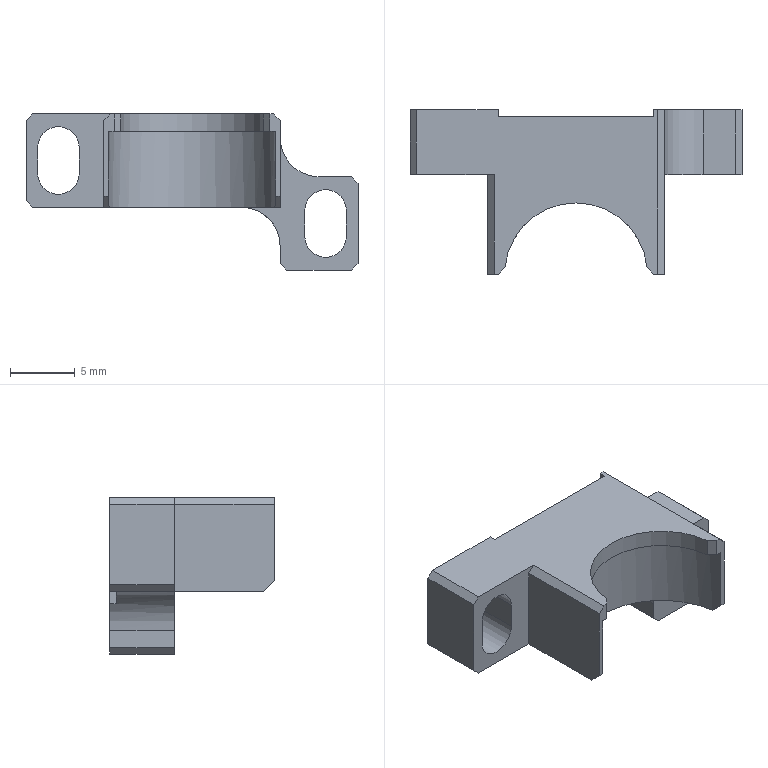Part | SolidWorks | features ICE 7, Chamfer 4, MoveFace 2, Extrusion 1, Fillet 1 | 1 solid | 42 faces | box 25.6 x 12.7 x 12.05 mm | volume 1054 mm3 | plane 34 | cylinder 8 | commonest cylinder face diameters 3.2 x4 6 x2 11 x1 12.9 x1
STEP:
#1=CARTESIAN_POINT('',(6.3,12.7,6.85));
#2=VERTEX_POINT('',#1);
#3=CARTESIAN_POINT('',(6.,12.7,6.85));
#4=VERTEX_POINT('',#3);
#5=CARTESIAN_POINT('',(0.,12.7,6.85));
#6=DIRECTION('',(-1.,0.,0.));
#7=VECTOR('',#6,1000.);
#8=LINE('',#5,#7);
#9=EDGE_CURVE('',#2,#4,#8,.T.);
#10=ORIENTED_EDGE('',*,*,#9,.F.);
#11=CARTESIAN_POINT('',(6.8,12.7,6.35));
#12=VERTEX_POINT('',#11);
#13=CARTESIAN_POINT('',(9.975,12.7,3.175));
#14=DIRECTION('',(0.7071,0.,-0.7071));
#15=VECTOR('',#14,1000.);
#16=LINE('',#13,#15);
#17=EDGE_CURVE('',#2,#12,#16,.T.);
#18=ORIENTED_EDGE('',*,*,#17,.T.);
#19=CARTESIAN_POINT('',(6.8,12.7,5.));
#20=VERTEX_POINT('',#19);
#21=CARTESIAN_POINT('',(6.8,12.7,0.));
#22=DIRECTION('',(0.,0.,1.));
#23=VECTOR('',#22,1000.);
#24=LINE('',#21,#23);
#25=EDGE_CURVE('',#20,#12,#24,.T.);
#26=ORIENTED_EDGE('',*,*,#25,.F.);
#27=CARTESIAN_POINT('',(9.8,12.7,2.));
#28=VERTEX_POINT('',#27);
#29=CARTESIAN_POINT('',(9.8,12.7,5.));
#30=DIRECTION('',(0.,-1.,0.));
#31=DIRECTION('',(-1.,0.,0.));
#32=AXIS2_PLACEMENT_3D('',#29,#30,#31);
#33=CIRCLE('',#32,3.);
#34=EDGE_CURVE('',#20,#28,#33,.T.);
#35=ORIENTED_EDGE('',*,*,#34,.T.);
#36=CARTESIAN_POINT('',(12.295,12.7,2.));
#37=VERTEX_POINT('',#36);
#38=CARTESIAN_POINT('',(6.8,12.7,2.));
#39=DIRECTION('',(1.,0.,0.));
#40=VECTOR('',#39,1000.);
#41=LINE('',#38,#40);
#42=EDGE_CURVE('',#28,#37,#41,.T.);
#43=ORIENTED_EDGE('',*,*,#42,.T.);
#44=CARTESIAN_POINT('',(12.8,12.7,1.495));
#45=VERTEX_POINT('',#44);
#46=CARTESIAN_POINT('',(10.547,12.7,3.747));
#47=DIRECTION('',(0.7071,0.,-0.7071));
#48=VECTOR('',#47,1000.);
#49=LINE('',#46,#48);
#50=EDGE_CURVE('',#37,#45,#49,.T.);
#51=ORIENTED_EDGE('',*,*,#50,.T.);
#52=CARTESIAN_POINT('',(12.8,12.7,-4.695));
#53=VERTEX_POINT('',#52);
#54=CARTESIAN_POINT('',(12.8,12.7,-5.2));
#55=DIRECTION('',(0.,0.,-1.));
#56=VECTOR('',#55,1000.);
#57=LINE('',#54,#56);
#58=EDGE_CURVE('',#45,#53,#57,.T.);
#59=ORIENTED_EDGE('',*,*,#58,.T.);
#60=CARTESIAN_POINT('',(12.295,12.7,-5.2));
#61=VERTEX_POINT('',#60);
#62=CARTESIAN_POINT('',(12.147,12.7,-5.347));
#63=DIRECTION('',(-0.7071,0.,-0.7071));
#64=VECTOR('',#63,1000.);
#65=LINE('',#62,#64);
#66=EDGE_CURVE('',#53,#61,#65,.T.);
#67=ORIENTED_EDGE('',*,*,#66,.T.);
#68=CARTESIAN_POINT('',(7.3,12.7,-5.2));
#69=VERTEX_POINT('',#68);
#70=CARTESIAN_POINT('',(6.8,12.7,-5.2));
#71=DIRECTION('',(-1.,0.,0.));
#72=VECTOR('',#71,1000.);
#73=LINE('',#70,#72);
#74=EDGE_CURVE('',#61,#69,#73,.T.);
#75=ORIENTED_EDGE('',*,*,#74,.T.);
#76=CARTESIAN_POINT('',(6.8,12.7,-4.7));
#77=VERTEX_POINT('',#76);
#78=CARTESIAN_POINT('',(4.45,12.7,-2.35));
#79=DIRECTION('',(-0.7071,0.,0.7071));
#80=VECTOR('',#79,1000.);
#81=LINE('',#78,#80);
#82=EDGE_CURVE('',#69,#77,#81,.T.);
#83=ORIENTED_EDGE('',*,*,#82,.T.);
#84=CARTESIAN_POINT('',(6.8,12.7,-3.35));
#85=VERTEX_POINT('',#84);
#86=CARTESIAN_POINT('',(6.8,12.7,-5.2));
#87=DIRECTION('',(0.,0.,1.));
#88=VECTOR('',#87,1000.);
#89=LINE('',#86,#88);
#90=EDGE_CURVE('',#77,#85,#89,.T.);
#91=ORIENTED_EDGE('',*,*,#90,.T.);
#92=CARTESIAN_POINT('',(6.,12.7,-1.31));
#93=VERTEX_POINT('',#92);
#94=CARTESIAN_POINT('',(3.8,12.7,-3.35));
#95=DIRECTION('',(0.,-1.,0.));
#96=DIRECTION('',(-1.,0.,0.));
#97=AXIS2_PLACEMENT_3D('',#94,#95,#96);
#98=CIRCLE('',#97,3.);
#99=EDGE_CURVE('',#85,#93,#98,.T.);
#100=ORIENTED_EDGE('',*,*,#99,.T.);
#101=CARTESIAN_POINT('',(6.,12.7,0.));
#102=DIRECTION('',(0.,0.,-1.));
#103=VECTOR('',#102,1000.);
#104=LINE('',#101,#103);
#105=EDGE_CURVE('',#4,#93,#104,.T.);
#106=ORIENTED_EDGE('',*,*,#105,.F.);
#107=EDGE_LOOP('',(#10,#18,#26,#35,#43,#51,#59,#67,#75,#83,#91,#100,#106));
#108=FACE_OUTER_BOUND('',#107,.T.);
#109=CARTESIAN_POINT('',(8.7,12.7,-2.6));
#110=VERTEX_POINT('',#109);
#111=CARTESIAN_POINT('',(11.9,12.7,-2.6));
#112=VERTEX_POINT('',#111);
#113=CARTESIAN_POINT('',(10.3,12.7,-2.6));
#114=DIRECTION('',(0.,-1.,0.));
#115=DIRECTION('',(1.,0.,0.));
#116=AXIS2_PLACEMENT_3D('',#113,#114,#115);
#117=CIRCLE('',#116,1.6);
#118=EDGE_CURVE('',#110,#112,#117,.T.);
#119=ORIENTED_EDGE('',*,*,#118,.T.);
#120=CARTESIAN_POINT('',(11.9,12.7,-0.6));
#121=VERTEX_POINT('',#120);
#122=CARTESIAN_POINT('',(11.9,12.7,-2.6));
#123=DIRECTION('',(0.,0.,1.));
#124=VECTOR('',#123,1000.);
#125=LINE('',#122,#124);
#126=EDGE_CURVE('',#112,#121,#125,.T.);
#127=ORIENTED_EDGE('',*,*,#126,.T.);
#128=CARTESIAN_POINT('',(8.7,12.7,-0.6));
#129=VERTEX_POINT('',#128);
#130=CARTESIAN_POINT('',(10.3,12.7,-0.6));
#131=DIRECTION('',(0.,-1.,0.));
#132=DIRECTION('',(1.,0.,0.));
#133=AXIS2_PLACEMENT_3D('',#130,#131,#132);
#134=CIRCLE('',#133,1.6);
#135=EDGE_CURVE('',#121,#129,#134,.T.);
#136=ORIENTED_EDGE('',*,*,#135,.T.);
#137=CARTESIAN_POINT('',(8.7,12.7,-2.6));
#138=DIRECTION('',(0.,0.,-1.));
#139=VECTOR('',#138,1000.);
#140=LINE('',#137,#139);
#141=EDGE_CURVE('',#129,#110,#140,.T.);
#142=ORIENTED_EDGE('',*,*,#141,.T.);
#143=EDGE_LOOP('',(#119,#127,#136,#142));
#144=FACE_BOUND('',#143,.T.);
#145=CARTESIAN_POINT('',(6.8,12.7,0.));
#146=DIRECTION('',(0.,1.,0.));
#147=DIRECTION('',(-1.,0.,0.));
#148=AXIS2_PLACEMENT_3D('',#145,#146,#147);
#149=PLANE('',#148);
#150=ADVANCED_FACE('',(#108,#144),#149,.T.);
#151=CARTESIAN_POINT('',(-6.8,0.,0.5));
#152=VERTEX_POINT('',#151);
#153=CARTESIAN_POINT('',(-6.8,0.,6.35));
#154=VERTEX_POINT('',#153);
#155=CARTESIAN_POINT('',(-6.8,0.,0.));
#156=DIRECTION('',(0.,0.,1.));
#157=VECTOR('',#156,1000.);
#158=LINE('',#155,#157);
#159=EDGE_CURVE('',#152,#154,#158,.T.);
#160=ORIENTED_EDGE('',*,*,#159,.T.);
#161=CARTESIAN_POINT('',(-6.8,7.7,6.35));
#162=VERTEX_POINT('',#161);
#163=CARTESIAN_POINT('',(-6.8,0.,6.35));
#164=DIRECTION('',(0.,1.,0.));
#165=VECTOR('',#164,1000.);
#166=LINE('',#163,#165);
#167=EDGE_CURVE('',#154,#162,#166,.T.);
#168=ORIENTED_EDGE('',*,*,#167,.T.);
#169=CARTESIAN_POINT('',(-6.8,7.7,-0.35));
#170=VERTEX_POINT('',#169);
#171=CARTESIAN_POINT('',(-6.8,7.7,6.5));
#172=DIRECTION('',(0.,0.,-1.));
#173=VECTOR('',#172,1000.);
#174=LINE('',#171,#173);
#175=EDGE_CURVE('',#162,#170,#174,.T.);
#176=ORIENTED_EDGE('',*,*,#175,.T.);
#177=CARTESIAN_POINT('',(-6.8,0.85,-0.35));
#178=VERTEX_POINT('',#177);
#179=CARTESIAN_POINT('',(-6.8,0.,-0.35));
#180=DIRECTION('',(0.,-1.,0.));
#181=VECTOR('',#180,1000.);
#182=LINE('',#179,#181);
#183=EDGE_CURVE('',#170,#178,#182,.T.);
#184=ORIENTED_EDGE('',*,*,#183,.T.);
#185=CARTESIAN_POINT('',(-6.8,0.25,0.25));
#186=DIRECTION('',(0.,-0.7071,0.7071));
#187=VECTOR('',#186,1000.);
#188=LINE('',#185,#187);
#189=EDGE_CURVE('',#178,#152,#188,.T.);
#190=ORIENTED_EDGE('',*,*,#189,.T.);
#191=EDGE_LOOP('',(#160,#168,#176,#184,#190));
#192=FACE_OUTER_BOUND('',#191,.T.);
#193=CARTESIAN_POINT('',(-6.8,0.,0.));
#194=DIRECTION('',(-1.,0.,0.));
#195=DIRECTION('',(0.,0.,1.));
#196=AXIS2_PLACEMENT_3D('',#193,#194,#195);
#197=PLANE('',#196);
#198=ADVANCED_FACE('',(#192),#197,.T.);
#199=CARTESIAN_POINT('',(5.475,0.5251,5.5));
#200=VERTEX_POINT('',#199);
#201=CARTESIAN_POINT('',(-5.475,0.5251,5.5));
#202=VERTEX_POINT('',#201);
#203=CARTESIAN_POINT('',(0.,0.,5.5));
#204=DIRECTION('',(0.,0.,1.));
#205=DIRECTION('',(-1.,0.,0.));
#206=AXIS2_PLACEMENT_3D('',#203,#204,#205);
#207=CIRCLE('',#206,5.5);
#208=EDGE_CURVE('',#200,#202,#207,.T.);
#209=ORIENTED_EDGE('',*,*,#208,.F.);
#210=CARTESIAN_POINT('',(5.475,0.5251,6.85));
#211=VERTEX_POINT('',#210);
#212=CARTESIAN_POINT('',(5.475,0.5251,10.));
#213=DIRECTION('',(0.,0.,1.));
#214=VECTOR('',#213,1000.);
#215=LINE('',#212,#214);
#216=EDGE_CURVE('',#200,#211,#215,.T.);
#217=ORIENTED_EDGE('',*,*,#216,.T.);
#218=CARTESIAN_POINT('',(-5.475,0.5251,6.85));
#219=VERTEX_POINT('',#218);
#220=CARTESIAN_POINT('',(0.,0.,6.85));
#221=DIRECTION('',(0.,0.,1.));
#222=DIRECTION('',(1.,0.,0.));
#223=AXIS2_PLACEMENT_3D('',#220,#221,#222);
#224=CIRCLE('',#223,5.5);
#225=EDGE_CURVE('',#211,#219,#224,.T.);
#226=ORIENTED_EDGE('',*,*,#225,.T.);
#227=CARTESIAN_POINT('',(-5.475,0.5251,10.));
#228=DIRECTION('',(0.,0.,-1.));
#229=VECTOR('',#228,1000.);
#230=LINE('',#227,#229);
#231=EDGE_CURVE('',#219,#202,#230,.T.);
#232=ORIENTED_EDGE('',*,*,#231,.T.);
#233=EDGE_LOOP('',(#209,#217,#226,#232));
#234=FACE_OUTER_BOUND('',#233,.T.);
#235=CARTESIAN_POINT('',(0.,0.,10.));
#236=DIRECTION('',(0.,0.,-1.));
#237=DIRECTION('',(-1.,0.,0.));
#238=AXIS2_PLACEMENT_3D('',#235,#236,#237);
#239=CYLINDRICAL_SURFACE('',#238,5.5);
#240=ADVANCED_FACE('',(#234),#239,.F.);
#241=CARTESIAN_POINT('',(-12.3,7.7,6.85));
#242=VERTEX_POINT('',#241);
#243=CARTESIAN_POINT('',(-6.3,7.7,6.85));
#244=VERTEX_POINT('',#243);
#245=CARTESIAN_POINT('',(0.,7.7,6.85));
#246=DIRECTION('',(1.,0.,0.));
#247=VECTOR('',#246,1000.);
#248=LINE('',#245,#247);
#249=EDGE_CURVE('',#242,#244,#248,.T.);
#250=ORIENTED_EDGE('',*,*,#249,.T.);
#251=CARTESIAN_POINT('',(-6.3,0.,6.85));
#252=VERTEX_POINT('',#251);
#253=CARTESIAN_POINT('',(-6.3,0.,6.85));
#254=DIRECTION('',(0.,-1.,0.));
#255=VECTOR('',#254,1000.);
#256=LINE('',#253,#255);
#257=EDGE_CURVE('',#244,#252,#256,.T.);
#258=ORIENTED_EDGE('',*,*,#257,.T.);
#259=CARTESIAN_POINT('',(-6.,0.,6.85));
#260=VERTEX_POINT('',#259);
#261=CARTESIAN_POINT('',(0.,0.,6.85));
#262=DIRECTION('',(-1.,0.,0.));
#263=VECTOR('',#262,1000.);
#264=LINE('',#261,#263);
#265=EDGE_CURVE('',#260,#252,#264,.T.);
#266=ORIENTED_EDGE('',*,*,#265,.F.);
#267=CARTESIAN_POINT('',(-3.,3.,6.85));
#268=DIRECTION('',(0.7071,0.7071,0.));
#269=VECTOR('',#268,1000.);
#270=LINE('',#267,#269);
#271=EDGE_CURVE('',#260,#219,#270,.T.);
#272=ORIENTED_EDGE('',*,*,#271,.T.);
#273=ORIENTED_EDGE('',*,*,#225,.F.);
#274=CARTESIAN_POINT('',(6.,0.,6.85));
#275=VERTEX_POINT('',#274);
#276=CARTESIAN_POINT('',(3.,3.,6.85));
#277=DIRECTION('',(0.7071,-0.7071,0.));
#278=VECTOR('',#277,1000.);
#279=LINE('',#276,#278);
#280=EDGE_CURVE('',#211,#275,#279,.T.);
#281=ORIENTED_EDGE('',*,*,#280,.T.);
#282=CARTESIAN_POINT('',(6.3,0.,6.85));
#283=VERTEX_POINT('',#282);
#284=CARTESIAN_POINT('',(0.,0.,6.85));
#285=DIRECTION('',(-1.,0.,0.));
#286=VECTOR('',#285,1000.);
#287=LINE('',#284,#286);
#288=EDGE_CURVE('',#283,#275,#287,.T.);
#289=ORIENTED_EDGE('',*,*,#288,.F.);
#290=CARTESIAN_POINT('',(6.3,0.,6.85));
#291=DIRECTION('',(0.,1.,0.));
#292=VECTOR('',#291,1000.);
#293=LINE('',#290,#292);
#294=EDGE_CURVE('',#283,#2,#293,.T.);
#295=ORIENTED_EDGE('',*,*,#294,.T.);
#296=ORIENTED_EDGE('',*,*,#9,.T.);
#297=CARTESIAN_POINT('',(6.,12.2,6.85));
#298=VERTEX_POINT('',#297);
#299=CARTESIAN_POINT('',(6.,0.,6.85));
#300=DIRECTION('',(0.,1.,0.));
#301=VECTOR('',#300,1000.);
#302=LINE('',#299,#301);
#303=EDGE_CURVE('',#298,#4,#302,.T.);
#304=ORIENTED_EDGE('',*,*,#303,.F.);
#305=CARTESIAN_POINT('',(-6.,12.2,6.85));
#306=VERTEX_POINT('',#305);
#307=CARTESIAN_POINT('',(0.,12.2,6.85));
#308=DIRECTION('',(1.,0.,0.));
#309=VECTOR('',#308,1000.);
#310=LINE('',#307,#309);
#311=EDGE_CURVE('',#306,#298,#310,.T.);
#312=ORIENTED_EDGE('',*,*,#311,.F.);
#313=CARTESIAN_POINT('',(-6.,12.7,6.85));
#314=VERTEX_POINT('',#313);
#315=CARTESIAN_POINT('',(-6.,12.2,6.85));
#316=DIRECTION('',(0.,1.,0.));
#317=VECTOR('',#316,1000.);
#318=LINE('',#315,#317);
#319=EDGE_CURVE('',#306,#314,#318,.T.);
#320=ORIENTED_EDGE('',*,*,#319,.T.);
#321=CARTESIAN_POINT('',(-12.3,12.7,6.85));
#322=VERTEX_POINT('',#321);
#323=CARTESIAN_POINT('',(0.,12.7,6.85));
#324=DIRECTION('',(-1.,0.,0.));
#325=VECTOR('',#324,1000.);
#326=LINE('',#323,#325);
#327=EDGE_CURVE('',#314,#322,#326,.T.);
#328=ORIENTED_EDGE('',*,*,#327,.T.);
#329=CARTESIAN_POINT('',(-12.3,0.,6.85));
#330=DIRECTION('',(0.,-1.,0.));
#331=VECTOR('',#330,1000.);
#332=LINE('',#329,#331);
#333=EDGE_CURVE('',#322,#242,#332,.T.);
#334=ORIENTED_EDGE('',*,*,#333,.T.);
#335=EDGE_LOOP('',(#250,#258,#266,#272,#273,#281,#289,#295,#296,#304,#312,#320,#328,#334));
#336=FACE_OUTER_BOUND('',#335,.T.);
#337=CARTESIAN_POINT('',(0.,0.,6.85));
#338=DIRECTION('',(0.,0.,1.));
#339=DIRECTION('',(1.,0.,0.));
#340=AXIS2_PLACEMENT_3D('',#337,#338,#339);
#341=PLANE('',#340);
#342=ADVANCED_FACE('',(#336),#341,.T.);
#343=CARTESIAN_POINT('',(-12.3,7.7,-0.35));
#344=VERTEX_POINT('',#343);
#345=CARTESIAN_POINT('',(0.,7.7,-0.35));
#346=DIRECTION('',(-1.,0.,0.));
#347=VECTOR('',#346,1000.);
#348=LINE('',#345,#347);
#349=EDGE_CURVE('',#170,#344,#348,.T.);
#350=ORIENTED_EDGE('',*,*,#349,.T.);
#351=CARTESIAN_POINT('',(-12.3,12.7,-0.35));
#352=VERTEX_POINT('',#351);
#353=CARTESIAN_POINT('',(-12.3,12.7,-0.35));
#354=DIRECTION('',(0.,1.,0.));
#355=VECTOR('',#354,1000.);
#356=LINE('',#353,#355);
#357=EDGE_CURVE('',#344,#352,#356,.T.);
#358=ORIENTED_EDGE('',*,*,#357,.T.);
#359=CARTESIAN_POINT('',(-6.,12.7,-0.35));
#360=VERTEX_POINT('',#359);
#361=CARTESIAN_POINT('',(0.,12.7,-0.35));
#362=DIRECTION('',(-1.,0.,0.));
#363=VECTOR('',#362,1000.);
#364=LINE('',#361,#363);
#365=EDGE_CURVE('',#360,#352,#364,.T.);
#366=ORIENTED_EDGE('',*,*,#365,.F.);
#367=CARTESIAN_POINT('',(-6.,12.2,-0.35));
#368=VERTEX_POINT('',#367);
#369=CARTESIAN_POINT('',(-6.,12.2,-0.35));
#370=DIRECTION('',(0.,1.,0.));
#371=VECTOR('',#370,1000.);
#372=LINE('',#369,#371);
#373=EDGE_CURVE('',#368,#360,#372,.T.);
#374=ORIENTED_EDGE('',*,*,#373,.F.);
#375=CARTESIAN_POINT('',(3.8,12.2,-0.35));
#376=VERTEX_POINT('',#375);
#377=CARTESIAN_POINT('',(0.,12.2,-0.35));
#378=DIRECTION('',(-1.,0.,0.));
#379=VECTOR('',#378,1000.);
#380=LINE('',#377,#379);
#381=EDGE_CURVE('',#376,#368,#380,.T.);
#382=ORIENTED_EDGE('',*,*,#381,.F.);
#383=CARTESIAN_POINT('',(3.8,7.7,-0.35));
#384=VERTEX_POINT('',#383);
#385=CARTESIAN_POINT('',(3.8,0.,-0.35));
#386=DIRECTION('',(0.,-1.,0.));
#387=VECTOR('',#386,1000.);
#388=LINE('',#385,#387);
#389=EDGE_CURVE('',#376,#384,#388,.T.);
#390=ORIENTED_EDGE('',*,*,#389,.T.);
#391=CARTESIAN_POINT('',(6.8,7.7,-0.35));
#392=VERTEX_POINT('',#391);
#393=CARTESIAN_POINT('',(0.,7.7,-0.35));
#394=DIRECTION('',(1.,0.,0.));
#395=VECTOR('',#394,1000.);
#396=LINE('',#393,#395);
#397=EDGE_CURVE('',#384,#392,#396,.T.);
#398=ORIENTED_EDGE('',*,*,#397,.T.);
#399=CARTESIAN_POINT('',(6.8,0.85,-0.35));
#400=VERTEX_POINT('',#399);
#401=CARTESIAN_POINT('',(6.8,0.,-0.35));
#402=DIRECTION('',(0.,1.,0.));
#403=VECTOR('',#402,1000.);
#404=LINE('',#401,#403);
#405=EDGE_CURVE('',#400,#392,#404,.T.);
#406=ORIENTED_EDGE('',*,*,#405,.F.);
#407=CARTESIAN_POINT('',(6.394,0.85,-0.35));
#408=VERTEX_POINT('',#407);
#409=CARTESIAN_POINT('',(-6.8,0.85,-0.35));
#410=DIRECTION('',(-1.,0.,0.));
#411=VECTOR('',#410,1000.);
#412=LINE('',#409,#411);
#413=EDGE_CURVE('',#400,#408,#412,.T.);
#414=ORIENTED_EDGE('',*,*,#413,.T.);
#415=CARTESIAN_POINT('',(-6.394,0.85,-0.35));
#416=VERTEX_POINT('',#415);
#417=CARTESIAN_POINT('',(0.,0.,-0.35));
#418=DIRECTION('',(0.,0.,-1.));
#419=DIRECTION('',(1.,0.,0.));
#420=AXIS2_PLACEMENT_3D('',#417,#418,#419);
#421=CIRCLE('',#420,6.45);
#422=EDGE_CURVE('',#416,#408,#421,.T.);
#423=ORIENTED_EDGE('',*,*,#422,.F.);
#424=CARTESIAN_POINT('',(-6.8,0.85,-0.35));
#425=DIRECTION('',(-1.,0.,0.));
#426=VECTOR('',#425,1000.);
#427=LINE('',#424,#426);
#428=EDGE_CURVE('',#416,#178,#427,.T.);
#429=ORIENTED_EDGE('',*,*,#428,.T.);
#430=ORIENTED_EDGE('',*,*,#183,.F.);
#431=EDGE_LOOP('',(#350,#358,#366,#374,#382,#390,#398,#406,#414,#423,#429,#430));
#432=FACE_OUTER_BOUND('',#431,.T.);
#433=CARTESIAN_POINT('',(0.,0.,-0.35));
#434=DIRECTION('',(0.,0.,1.));
#435=DIRECTION('',(1.,0.,0.));
#436=AXIS2_PLACEMENT_3D('',#433,#434,#435);
#437=PLANE('',#436);
#438=ADVANCED_FACE('',(#432),#437,.F.);
#439=CARTESIAN_POINT('',(6.,0.,5.5));
#440=VERTEX_POINT('',#439);
#441=CARTESIAN_POINT('',(6.45,0.,5.5));
#442=VERTEX_POINT('',#441);
#443=CARTESIAN_POINT('',(0.,0.,5.5));
#444=DIRECTION('',(1.,0.,0.));
#445=VECTOR('',#444,1000.);
#446=LINE('',#443,#445);
#447=EDGE_CURVE('',#440,#442,#446,.T.);
#448=ORIENTED_EDGE('',*,*,#447,.F.);
#449=CARTESIAN_POINT('',(3.,3.,5.5));
#450=DIRECTION('',(-0.7071,0.7071,0.));
#451=VECTOR('',#450,1000.);
#452=LINE('',#449,#451);
#453=EDGE_CURVE('',#440,#200,#452,.T.);
#454=ORIENTED_EDGE('',*,*,#453,.T.);
#455=ORIENTED_EDGE('',*,*,#208,.T.);
#456=CARTESIAN_POINT('',(-6.,0.,5.5));
#457=VERTEX_POINT('',#456);
#458=CARTESIAN_POINT('',(-3.,3.,5.5));
#459=DIRECTION('',(-0.7071,-0.7071,0.));
#460=VECTOR('',#459,1000.);
#461=LINE('',#458,#460);
#462=EDGE_CURVE('',#202,#457,#461,.T.);
#463=ORIENTED_EDGE('',*,*,#462,.T.);
#464=CARTESIAN_POINT('',(-6.45,0.,5.5));
#465=VERTEX_POINT('',#464);
#466=CARTESIAN_POINT('',(0.,0.,5.5));
#467=DIRECTION('',(1.,0.,0.));
#468=VECTOR('',#467,1000.);
#469=LINE('',#466,#468);
#470=EDGE_CURVE('',#465,#457,#469,.T.);
#471=ORIENTED_EDGE('',*,*,#470,.F.);
#472=CARTESIAN_POINT('',(0.,0.,5.5));
#473=DIRECTION('',(0.,0.,-1.));
#474=DIRECTION('',(-1.,0.,0.));
#475=AXIS2_PLACEMENT_3D('',#472,#473,#474);
#476=CIRCLE('',#475,6.45);
#477=EDGE_CURVE('',#465,#442,#476,.T.);
#478=ORIENTED_EDGE('',*,*,#477,.T.);
#479=EDGE_LOOP('',(#448,#454,#455,#463,#471,#478));
#480=FACE_OUTER_BOUND('',#479,.T.);
#481=CARTESIAN_POINT('',(0.,0.,5.5));
#482=DIRECTION('',(0.,0.,-1.));
#483=DIRECTION('',(-1.,0.,0.));
#484=AXIS2_PLACEMENT_3D('',#481,#482,#483);
#485=PLANE('',#484);
#486=ADVANCED_FACE('',(#480),#485,.T.);
#487=ORIENTED_EDGE('',*,*,#422,.T.);
#488=CARTESIAN_POINT('',(6.45,0.,0.5));
#489=VERTEX_POINT('',#488);
#490=CARTESIAN_POINT('',(6.394,0.85,-0.35));
#491=CARTESIAN_POINT('',(6.431,0.5681,-0.06811));
#492=CARTESIAN_POINT('',(6.45,0.2844,0.2156));
#493=CARTESIAN_POINT('',(6.45,0.,0.5));
#494=(BOUNDED_CURVE()B_SPLINE_CURVE(3,(#490,#491,#492,#493),.UNSPECIFIED.,.F.,.F.)B_SPLINE_CURVE_WITH_KNOTS((4,4),(1.439,1.571),.UNSPECIFIED.)CURVE()GEOMETRIC_REPRESENTATION_ITEM()RATIONAL_B_SPLINE_CURVE((1.,0.9985,0.9985,1.))REPRESENTATION_ITEM(''));
#495=EDGE_CURVE('',#408,#489,#494,.T.);
#496=ORIENTED_EDGE('',*,*,#495,.T.);
#497=CARTESIAN_POINT('',(6.45,0.,5.5));
#498=DIRECTION('',(0.,0.,1.));
#499=VECTOR('',#498,1000.);
#500=LINE('',#497,#499);
#501=EDGE_CURVE('',#489,#442,#500,.T.);
#502=ORIENTED_EDGE('',*,*,#501,.T.);
#503=ORIENTED_EDGE('',*,*,#477,.F.);
#504=CARTESIAN_POINT('',(-6.45,0.,0.5));
#505=VERTEX_POINT('',#504);
#506=CARTESIAN_POINT('',(-6.45,0.,5.5));
#507=DIRECTION('',(0.,0.,-1.));
#508=VECTOR('',#507,1000.);
#509=LINE('',#506,#508);
#510=EDGE_CURVE('',#465,#505,#509,.T.);
#511=ORIENTED_EDGE('',*,*,#510,.T.);
#512=CARTESIAN_POINT('',(-6.45,0.,0.5));
#513=CARTESIAN_POINT('',(-6.45,0.2844,0.2156));
#514=CARTESIAN_POINT('',(-6.431,0.5681,-0.06811));
#515=CARTESIAN_POINT('',(-6.394,0.85,-0.35));
#516=(BOUNDED_CURVE()B_SPLINE_CURVE(3,(#512,#513,#514,#515),.UNSPECIFIED.,.F.,.F.)B_SPLINE_CURVE_WITH_KNOTS((4,4),(4.712,4.845),.UNSPECIFIED.)CURVE()GEOMETRIC_REPRESENTATION_ITEM()RATIONAL_B_SPLINE_CURVE((1.,0.9985,0.9985,1.))REPRESENTATION_ITEM(''));
#517=EDGE_CURVE('',#505,#416,#516,.T.);
#518=ORIENTED_EDGE('',*,*,#517,.T.);
#519=EDGE_LOOP('',(#487,#496,#502,#503,#511,#518));
#520=FACE_OUTER_BOUND('',#519,.T.);
#521=CARTESIAN_POINT('',(0.,0.,5.5));
#522=DIRECTION('',(0.,0.,-1.));
#523=DIRECTION('',(-1.,0.,0.));
#524=AXIS2_PLACEMENT_3D('',#521,#522,#523);
#525=CYLINDRICAL_SURFACE('',#524,6.45);
#526=ADVANCED_FACE('',(#520),#525,.F.);
#527=CARTESIAN_POINT('',(-12.8,12.7,0.15));
#528=VERTEX_POINT('',#527);
#529=CARTESIAN_POINT('',(-12.8,12.7,6.35));
#530=VERTEX_POINT('',#529);
#531=CARTESIAN_POINT('',(-12.8,12.7,6.5));
#532=DIRECTION('',(0.,0.,1.));
#533=VECTOR('',#532,1000.);
#534=LINE('',#531,#533);
#535=EDGE_CURVE('',#528,#530,#534,.T.);
#536=ORIENTED_EDGE('',*,*,#535,.T.);
#537=CARTESIAN_POINT('',(-6.175,12.7,12.975));
#538=DIRECTION('',(0.7071,0.,0.7071));
#539=VECTOR('',#538,1000.);
#540=LINE('',#537,#539);
#541=EDGE_CURVE('',#530,#322,#540,.T.);
#542=ORIENTED_EDGE('',*,*,#541,.T.);
#543=ORIENTED_EDGE('',*,*,#327,.F.);
#544=CARTESIAN_POINT('',(-6.,12.7,6.5));
#545=DIRECTION('',(0.,0.,1.));
#546=VECTOR('',#545,1000.);
#547=LINE('',#544,#546);
#548=EDGE_CURVE('',#360,#314,#547,.T.);
#549=ORIENTED_EDGE('',*,*,#548,.F.);
#550=ORIENTED_EDGE('',*,*,#365,.T.);
#551=CARTESIAN_POINT('',(-2.925,12.7,-9.725));
#552=DIRECTION('',(-0.7071,0.,0.7071));
#553=VECTOR('',#552,1000.);
#554=LINE('',#551,#553);
#555=EDGE_CURVE('',#352,#528,#554,.T.);
#556=ORIENTED_EDGE('',*,*,#555,.T.);
#557=EDGE_LOOP('',(#536,#542,#543,#549,#550,#556));
#558=FACE_OUTER_BOUND('',#557,.T.);
#559=CARTESIAN_POINT('',(-8.7,12.7,4.25));
#560=VERTEX_POINT('',#559);
#561=CARTESIAN_POINT('',(-11.9,12.7,4.25));
#562=VERTEX_POINT('',#561);
#563=CARTESIAN_POINT('',(-10.3,12.7,4.25));
#564=DIRECTION('',(0.,-1.,0.));
#565=DIRECTION('',(-1.,0.,0.));
#566=AXIS2_PLACEMENT_3D('',#563,#564,#565);
#567=CIRCLE('',#566,1.6);
#568=EDGE_CURVE('',#560,#562,#567,.T.);
#569=ORIENTED_EDGE('',*,*,#568,.T.);
#570=CARTESIAN_POINT('',(-11.9,12.7,2.25));
#571=VERTEX_POINT('',#570);
#572=CARTESIAN_POINT('',(-11.9,12.7,2.25));
#573=DIRECTION('',(0.,0.,-1.));
#574=VECTOR('',#573,1000.);
#575=LINE('',#572,#574);
#576=EDGE_CURVE('',#562,#571,#575,.T.);
#577=ORIENTED_EDGE('',*,*,#576,.T.);
#578=CARTESIAN_POINT('',(-8.7,12.7,2.25));
#579=VERTEX_POINT('',#578);
#580=CARTESIAN_POINT('',(-10.3,12.7,2.25));
#581=DIRECTION('',(0.,-1.,0.));
#582=DIRECTION('',(-1.,0.,0.));
#583=AXIS2_PLACEMENT_3D('',#580,#581,#582);
#584=CIRCLE('',#583,1.6);
#585=EDGE_CURVE('',#571,#579,#584,.T.);
#586=ORIENTED_EDGE('',*,*,#585,.T.);
#587=CARTESIAN_POINT('',(-8.7,12.7,2.25));
#588=DIRECTION('',(0.,0.,1.));
#589=VECTOR('',#588,1000.);
#590=LINE('',#587,#589);
#591=EDGE_CURVE('',#579,#560,#590,.T.);
#592=ORIENTED_EDGE('',*,*,#591,.T.);
#593=EDGE_LOOP('',(#569,#577,#586,#592));
#594=FACE_BOUND('',#593,.T.);
#595=CARTESIAN_POINT('',(6.8,12.7,0.));
#596=DIRECTION('',(0.,1.,0.));
#597=DIRECTION('',(-1.,0.,0.));
#598=AXIS2_PLACEMENT_3D('',#595,#596,#597);
#599=PLANE('',#598);
#600=ADVANCED_FACE('',(#558,#594),#599,.T.);
#601=ORIENTED_EDGE('',*,*,#25,.T.);
#602=CARTESIAN_POINT('',(6.8,0.,6.35));
#603=VERTEX_POINT('',#602);
#604=CARTESIAN_POINT('',(6.8,0.,6.35));
#605=DIRECTION('',(0.,-1.,0.));
#606=VECTOR('',#605,1000.);
#607=LINE('',#604,#606);
#608=EDGE_CURVE('',#12,#603,#607,.T.);
#609=ORIENTED_EDGE('',*,*,#608,.T.);
#610=CARTESIAN_POINT('',(6.8,0.,0.5));
#611=VERTEX_POINT('',#610);
#612=CARTESIAN_POINT('',(6.8,0.,0.));
#613=DIRECTION('',(0.,0.,1.));
#614=VECTOR('',#613,1000.);
#615=LINE('',#612,#614);
#616=EDGE_CURVE('',#611,#603,#615,.T.);
#617=ORIENTED_EDGE('',*,*,#616,.F.);
#618=CARTESIAN_POINT('',(6.8,0.25,0.25));
#619=DIRECTION('',(0.,0.7071,-0.7071));
#620=VECTOR('',#619,1000.);
#621=LINE('',#618,#620);
#622=EDGE_CURVE('',#611,#400,#621,.T.);
#623=ORIENTED_EDGE('',*,*,#622,.T.);
#624=ORIENTED_EDGE('',*,*,#405,.T.);
#625=CARTESIAN_POINT('',(6.8,7.7,5.));
#626=VERTEX_POINT('',#625);
#627=CARTESIAN_POINT('',(6.8,7.7,0.));
#628=DIRECTION('',(0.,0.,1.));
#629=VECTOR('',#628,1000.);
#630=LINE('',#627,#629);
#631=EDGE_CURVE('',#392,#626,#630,.T.);
#632=ORIENTED_EDGE('',*,*,#631,.T.);
#633=CARTESIAN_POINT('',(6.8,12.7,5.));
#634=DIRECTION('',(0.,1.,0.));
#635=VECTOR('',#634,1000.);
#636=LINE('',#633,#635);
#637=EDGE_CURVE('',#626,#20,#636,.T.);
#638=ORIENTED_EDGE('',*,*,#637,.T.);
#639=EDGE_LOOP('',(#601,#609,#617,#623,#624,#632,#638));
#640=FACE_OUTER_BOUND('',#639,.T.);
#641=CARTESIAN_POINT('',(6.8,0.,0.));
#642=DIRECTION('',(1.,0.,0.));
#643=DIRECTION('',(0.,0.,-1.));
#644=AXIS2_PLACEMENT_3D('',#641,#642,#643);
#645=PLANE('',#644);
#646=ADVANCED_FACE('',(#640),#645,.T.);
#647=ORIENTED_EDGE('',*,*,#90,.F.);
#648=CARTESIAN_POINT('',(6.8,7.7,-4.7));
#649=VERTEX_POINT('',#648);
#650=CARTESIAN_POINT('',(6.8,7.7,-4.7));
#651=DIRECTION('',(0.,-1.,0.));
#652=VECTOR('',#651,1000.);
#653=LINE('',#650,#652);
#654=EDGE_CURVE('',#77,#649,#653,.T.);
#655=ORIENTED_EDGE('',*,*,#654,.T.);
#656=CARTESIAN_POINT('',(6.8,7.7,-3.35));
#657=VERTEX_POINT('',#656);
#658=CARTESIAN_POINT('',(6.8,7.7,-5.2));
#659=DIRECTION('',(0.,0.,1.));
#660=VECTOR('',#659,1000.);
#661=LINE('',#658,#660);
#662=EDGE_CURVE('',#649,#657,#661,.T.);
#663=ORIENTED_EDGE('',*,*,#662,.T.);
#664=CARTESIAN_POINT('',(6.8,7.7,-3.35));
#665=DIRECTION('',(0.,1.,0.));
#666=VECTOR('',#665,1000.);
#667=LINE('',#664,#666);
#668=EDGE_CURVE('',#657,#85,#667,.T.);
#669=ORIENTED_EDGE('',*,*,#668,.T.);
#670=EDGE_LOOP('',(#647,#655,#663,#669));
#671=FACE_OUTER_BOUND('',#670,.T.);
#672=CARTESIAN_POINT('',(6.8,7.7,-5.2));
#673=DIRECTION('',(-1.,0.,0.));
#674=DIRECTION('',(0.,-1.,0.));
#675=AXIS2_PLACEMENT_3D('',#672,#673,#674);
#676=PLANE('',#675);
#677=ADVANCED_FACE('',(#671),#676,.T.);
#678=CARTESIAN_POINT('',(12.295,7.7,-5.2));
#679=VERTEX_POINT('',#678);
#680=CARTESIAN_POINT('',(7.3,7.7,-5.2));
#681=VERTEX_POINT('',#680);
#682=CARTESIAN_POINT('',(6.8,7.7,-5.2));
#683=DIRECTION('',(-1.,0.,0.));
#684=VECTOR('',#683,1000.);
#685=LINE('',#682,#684);
#686=EDGE_CURVE('',#679,#681,#685,.T.);
#687=ORIENTED_EDGE('',*,*,#686,.T.);
#688=CARTESIAN_POINT('',(7.3,7.7,-5.2));
#689=DIRECTION('',(0.,1.,0.));
#690=VECTOR('',#689,1000.);
#691=LINE('',#688,#690);
#692=EDGE_CURVE('',#681,#69,#691,.T.);
#693=ORIENTED_EDGE('',*,*,#692,.T.);
#694=ORIENTED_EDGE('',*,*,#74,.F.);
#695=CARTESIAN_POINT('',(12.295,7.7,-5.2));
#696=DIRECTION('',(0.,-1.,0.));
#697=VECTOR('',#696,1000.);
#698=LINE('',#695,#697);
#699=EDGE_CURVE('',#61,#679,#698,.T.);
#700=ORIENTED_EDGE('',*,*,#699,.T.);
#701=EDGE_LOOP('',(#687,#693,#694,#700));
#702=FACE_OUTER_BOUND('',#701,.T.);
#703=CARTESIAN_POINT('',(6.8,7.7,-5.2));
#704=DIRECTION('',(0.,0.,-1.));
#705=DIRECTION('',(-1.,0.,0.));
#706=AXIS2_PLACEMENT_3D('',#703,#704,#705);
#707=PLANE('',#706);
#708=ADVANCED_FACE('',(#702),#707,.T.);
#709=CARTESIAN_POINT('',(12.8,7.7,1.495));
#710=VERTEX_POINT('',#709);
#711=CARTESIAN_POINT('',(12.8,7.7,-4.695));
#712=VERTEX_POINT('',#711);
#713=CARTESIAN_POINT('',(12.8,7.7,-5.2));
#714=DIRECTION('',(0.,0.,-1.));
#715=VECTOR('',#714,1000.);
#716=LINE('',#713,#715);
#717=EDGE_CURVE('',#710,#712,#716,.T.);
#718=ORIENTED_EDGE('',*,*,#717,.T.);
#719=CARTESIAN_POINT('',(12.8,7.7,-4.695));
#720=DIRECTION('',(0.,1.,0.));
#721=VECTOR('',#720,1000.);
#722=LINE('',#719,#721);
#723=EDGE_CURVE('',#712,#53,#722,.T.);
#724=ORIENTED_EDGE('',*,*,#723,.T.);
#725=ORIENTED_EDGE('',*,*,#58,.F.);
#726=CARTESIAN_POINT('',(12.8,7.7,1.495));
#727=DIRECTION('',(0.,-1.,0.));
#728=VECTOR('',#727,1000.);
#729=LINE('',#726,#728);
#730=EDGE_CURVE('',#45,#710,#729,.T.);
#731=ORIENTED_EDGE('',*,*,#730,.T.);
#732=EDGE_LOOP('',(#718,#724,#725,#731));
#733=FACE_OUTER_BOUND('',#732,.T.);
#734=CARTESIAN_POINT('',(12.8,7.7,-5.2));
#735=DIRECTION('',(1.,0.,0.));
#736=DIRECTION('',(0.,1.,0.));
#737=AXIS2_PLACEMENT_3D('',#734,#735,#736);
#738=PLANE('',#737);
#739=ADVANCED_FACE('',(#733),#738,.T.);
#740=ORIENTED_EDGE('',*,*,#42,.F.);
#741=CARTESIAN_POINT('',(9.8,7.7,2.));
#742=VERTEX_POINT('',#741);
#743=CARTESIAN_POINT('',(9.8,7.7,2.));
#744=DIRECTION('',(0.,-1.,0.));
#745=VECTOR('',#744,1000.);
#746=LINE('',#743,#745);
#747=EDGE_CURVE('',#28,#742,#746,.T.);
#748=ORIENTED_EDGE('',*,*,#747,.T.);
#749=CARTESIAN_POINT('',(12.295,7.7,2.));
#750=VERTEX_POINT('',#749);
#751=CARTESIAN_POINT('',(6.8,7.7,2.));
#752=DIRECTION('',(1.,0.,0.));
#753=VECTOR('',#752,1000.);
#754=LINE('',#751,#753);
#755=EDGE_CURVE('',#742,#750,#754,.T.);
#756=ORIENTED_EDGE('',*,*,#755,.T.);
#757=CARTESIAN_POINT('',(12.295,7.7,2.));
#758=DIRECTION('',(0.,1.,0.));
#759=VECTOR('',#758,1000.);
#760=LINE('',#757,#759);
#761=EDGE_CURVE('',#750,#37,#760,.T.);
#762=ORIENTED_EDGE('',*,*,#761,.T.);
#763=EDGE_LOOP('',(#740,#748,#756,#762));
#764=FACE_OUTER_BOUND('',#763,.T.);
#765=CARTESIAN_POINT('',(6.8,7.7,2.));
#766=DIRECTION('',(0.,0.,1.));
#767=DIRECTION('',(1.,0.,0.));
#768=AXIS2_PLACEMENT_3D('',#765,#766,#767);
#769=PLANE('',#768);
#770=ADVANCED_FACE('',(#764),#769,.T.);
#771=CARTESIAN_POINT('',(11.9,7.7,-2.6));
#772=VERTEX_POINT('',#771);
#773=CARTESIAN_POINT('',(11.9,7.7,-0.6));
#774=VERTEX_POINT('',#773);
#775=CARTESIAN_POINT('',(11.9,7.7,-2.6));
#776=DIRECTION('',(0.,0.,1.));
#777=VECTOR('',#776,1000.);
#778=LINE('',#775,#777);
#779=EDGE_CURVE('',#772,#774,#778,.T.);
#780=ORIENTED_EDGE('',*,*,#779,.F.);
#781=CARTESIAN_POINT('',(8.7,7.7,-2.6));
#782=VERTEX_POINT('',#781);
#783=CARTESIAN_POINT('',(10.3,7.7,-2.6));
#784=DIRECTION('',(0.,-1.,0.));
#785=DIRECTION('',(1.,0.,0.));
#786=AXIS2_PLACEMENT_3D('',#783,#784,#785);
#787=CIRCLE('',#786,1.6);
#788=EDGE_CURVE('',#782,#772,#787,.T.);
#789=ORIENTED_EDGE('',*,*,#788,.F.);
#790=CARTESIAN_POINT('',(8.7,7.7,-0.6));
#791=VERTEX_POINT('',#790);
#792=CARTESIAN_POINT('',(8.7,7.7,-2.6));
#793=DIRECTION('',(0.,0.,-1.));
#794=VECTOR('',#793,1000.);
#795=LINE('',#792,#794);
#796=EDGE_CURVE('',#791,#782,#795,.T.);
#797=ORIENTED_EDGE('',*,*,#796,.F.);
#798=CARTESIAN_POINT('',(10.3,7.7,-0.6));
#799=DIRECTION('',(0.,-1.,0.));
#800=DIRECTION('',(1.,0.,0.));
#801=AXIS2_PLACEMENT_3D('',#798,#799,#800);
#802=CIRCLE('',#801,1.6);
#803=EDGE_CURVE('',#774,#791,#802,.T.);
#804=ORIENTED_EDGE('',*,*,#803,.F.);
#805=EDGE_LOOP('',(#780,#789,#797,#804));
#806=FACE_BOUND('',#805,.T.);
#807=ORIENTED_EDGE('',*,*,#662,.F.);
#808=CARTESIAN_POINT('',(7.3,7.7,-5.2));
#809=DIRECTION('',(0.7071,0.,-0.7071));
#810=VECTOR('',#809,1000.);
#811=LINE('',#808,#810);
#812=EDGE_CURVE('',#649,#681,#811,.T.);
#813=ORIENTED_EDGE('',*,*,#812,.T.);
#814=ORIENTED_EDGE('',*,*,#686,.F.);
#815=CARTESIAN_POINT('',(13.047,7.7,-4.447));
#816=DIRECTION('',(0.7071,0.,0.7071));
#817=VECTOR('',#816,1000.);
#818=LINE('',#815,#817);
#819=EDGE_CURVE('',#679,#712,#818,.T.);
#820=ORIENTED_EDGE('',*,*,#819,.T.);
#821=ORIENTED_EDGE('',*,*,#717,.F.);
#822=CARTESIAN_POINT('',(12.047,7.7,2.247));
#823=DIRECTION('',(-0.7071,0.,0.7071));
#824=VECTOR('',#823,1000.);
#825=LINE('',#822,#824);
#826=EDGE_CURVE('',#710,#750,#825,.T.);
#827=ORIENTED_EDGE('',*,*,#826,.T.);
#828=ORIENTED_EDGE('',*,*,#755,.F.);
#829=CARTESIAN_POINT('',(9.8,7.7,5.));
#830=DIRECTION('',(0.,1.,0.));
#831=DIRECTION('',(-1.,0.,0.));
#832=AXIS2_PLACEMENT_3D('',#829,#830,#831);
#833=CIRCLE('',#832,3.);
#834=EDGE_CURVE('',#742,#626,#833,.T.);
#835=ORIENTED_EDGE('',*,*,#834,.T.);
#836=ORIENTED_EDGE('',*,*,#631,.F.);
#837=ORIENTED_EDGE('',*,*,#397,.F.);
#838=CARTESIAN_POINT('',(3.8,7.7,-3.35));
#839=DIRECTION('',(0.,1.,0.));
#840=DIRECTION('',(-1.,0.,0.));
#841=AXIS2_PLACEMENT_3D('',#838,#839,#840);
#842=CIRCLE('',#841,3.);
#843=EDGE_CURVE('',#384,#657,#842,.T.);
#844=ORIENTED_EDGE('',*,*,#843,.T.);
#845=EDGE_LOOP('',(#807,#813,#814,#820,#821,#827,#828,#835,#836,#837,#844));
#846=FACE_OUTER_BOUND('',#845,.T.);
#847=CARTESIAN_POINT('',(0.,7.7,0.));
#848=DIRECTION('',(0.,1.,0.));
#849=DIRECTION('',(-1.,0.,0.));
#850=AXIS2_PLACEMENT_3D('',#847,#848,#849);
#851=PLANE('',#850);
#852=ADVANCED_FACE('',(#806,#846),#851,.F.);
#853=CARTESIAN_POINT('',(-12.8,7.7,0.15));
#854=VERTEX_POINT('',#853);
#855=CARTESIAN_POINT('',(-12.8,7.7,6.35));
#856=VERTEX_POINT('',#855);
#857=CARTESIAN_POINT('',(-12.8,7.7,6.5));
#858=DIRECTION('',(0.,0.,1.));
#859=VECTOR('',#858,1000.);
#860=LINE('',#857,#859);
#861=EDGE_CURVE('',#854,#856,#860,.T.);
#862=ORIENTED_EDGE('',*,*,#861,.T.);
#863=CARTESIAN_POINT('',(-12.8,7.7,6.35));
#864=DIRECTION('',(0.,1.,0.));
#865=VECTOR('',#864,1000.);
#866=LINE('',#863,#865);
#867=EDGE_CURVE('',#856,#530,#866,.T.);
#868=ORIENTED_EDGE('',*,*,#867,.T.);
#869=ORIENTED_EDGE('',*,*,#535,.F.);
#870=CARTESIAN_POINT('',(-12.8,7.7,0.15));
#871=DIRECTION('',(0.,-1.,0.));
#872=VECTOR('',#871,1000.);
#873=LINE('',#870,#872);
#874=EDGE_CURVE('',#528,#854,#873,.T.);
#875=ORIENTED_EDGE('',*,*,#874,.T.);
#876=EDGE_LOOP('',(#862,#868,#869,#875));
#877=FACE_OUTER_BOUND('',#876,.T.);
#878=CARTESIAN_POINT('',(-12.8,7.7,6.5));
#879=DIRECTION('',(-1.,0.,0.));
#880=DIRECTION('',(0.,-1.,0.));
#881=AXIS2_PLACEMENT_3D('',#878,#879,#880);
#882=PLANE('',#881);
#883=ADVANCED_FACE('',(#877),#882,.T.);
#884=CARTESIAN_POINT('',(-11.9,7.7,4.25));
#885=VERTEX_POINT('',#884);
#886=CARTESIAN_POINT('',(-11.9,7.7,2.25));
#887=VERTEX_POINT('',#886);
#888=CARTESIAN_POINT('',(-11.9,7.7,2.25));
#889=DIRECTION('',(0.,0.,-1.));
#890=VECTOR('',#889,1000.);
#891=LINE('',#888,#890);
#892=EDGE_CURVE('',#885,#887,#891,.T.);
#893=ORIENTED_EDGE('',*,*,#892,.F.);
#894=CARTESIAN_POINT('',(-8.7,7.7,4.25));
#895=VERTEX_POINT('',#894);
#896=CARTESIAN_POINT('',(-10.3,7.7,4.25));
#897=DIRECTION('',(0.,-1.,0.));
#898=DIRECTION('',(-1.,0.,0.));
#899=AXIS2_PLACEMENT_3D('',#896,#897,#898);
#900=CIRCLE('',#899,1.6);
#901=EDGE_CURVE('',#895,#885,#900,.T.);
#902=ORIENTED_EDGE('',*,*,#901,.F.);
#903=CARTESIAN_POINT('',(-8.7,7.7,2.25));
#904=VERTEX_POINT('',#903);
#905=CARTESIAN_POINT('',(-8.7,7.7,2.25));
#906=DIRECTION('',(0.,0.,1.));
#907=VECTOR('',#906,1000.);
#908=LINE('',#905,#907);
#909=EDGE_CURVE('',#904,#895,#908,.T.);
#910=ORIENTED_EDGE('',*,*,#909,.F.);
#911=CARTESIAN_POINT('',(-10.3,7.7,2.25));
#912=DIRECTION('',(0.,-1.,0.));
#913=DIRECTION('',(-1.,0.,0.));
#914=AXIS2_PLACEMENT_3D('',#911,#912,#913);
#915=CIRCLE('',#914,1.6);
#916=EDGE_CURVE('',#887,#904,#915,.T.);
#917=ORIENTED_EDGE('',*,*,#916,.F.);
#918=EDGE_LOOP('',(#893,#902,#910,#917));
#919=FACE_BOUND('',#918,.T.);
#920=ORIENTED_EDGE('',*,*,#249,.F.);
#921=CARTESIAN_POINT('',(-12.8,7.7,6.35));
#922=DIRECTION('',(-0.7071,0.,-0.7071));
#923=VECTOR('',#922,1000.);
#924=LINE('',#921,#923);
#925=EDGE_CURVE('',#242,#856,#924,.T.);
#926=ORIENTED_EDGE('',*,*,#925,.T.);
#927=ORIENTED_EDGE('',*,*,#861,.F.);
#928=CARTESIAN_POINT('',(-12.3,7.7,-0.35));
#929=DIRECTION('',(0.7071,0.,-0.7071));
#930=VECTOR('',#929,1000.);
#931=LINE('',#928,#930);
#932=EDGE_CURVE('',#854,#344,#931,.T.);
#933=ORIENTED_EDGE('',*,*,#932,.T.);
#934=ORIENTED_EDGE('',*,*,#349,.F.);
#935=ORIENTED_EDGE('',*,*,#175,.F.);
#936=CARTESIAN_POINT('',(-6.575,7.7,6.575));
#937=DIRECTION('',(0.7071,0.,0.7071));
#938=VECTOR('',#937,1000.);
#939=LINE('',#936,#938);
#940=EDGE_CURVE('',#162,#244,#939,.T.);
#941=ORIENTED_EDGE('',*,*,#940,.T.);
#942=EDGE_LOOP('',(#920,#926,#927,#933,#934,#935,#941));
#943=FACE_OUTER_BOUND('',#942,.T.);
#944=CARTESIAN_POINT('',(0.,7.7,0.));
#945=DIRECTION('',(0.,1.,0.));
#946=DIRECTION('',(-1.,0.,0.));
#947=AXIS2_PLACEMENT_3D('',#944,#945,#946);
#948=PLANE('',#947);
#949=ADVANCED_FACE('',(#919,#943),#948,.F.);
#950=ORIENTED_EDGE('',*,*,#901,.T.);
#951=CARTESIAN_POINT('',(-11.9,12.7,4.25));
#952=DIRECTION('',(0.,-1.,0.));
#953=VECTOR('',#952,1000.);
#954=LINE('',#951,#953);
#955=EDGE_CURVE('',#562,#885,#954,.T.);
#956=ORIENTED_EDGE('',*,*,#955,.F.);
#957=ORIENTED_EDGE('',*,*,#568,.F.);
#958=CARTESIAN_POINT('',(-8.7,12.7,4.25));
#959=DIRECTION('',(0.,-1.,0.));
#960=VECTOR('',#959,1000.);
#961=LINE('',#958,#960);
#962=EDGE_CURVE('',#560,#895,#961,.T.);
#963=ORIENTED_EDGE('',*,*,#962,.T.);
#964=EDGE_LOOP('',(#950,#956,#957,#963));
#965=FACE_OUTER_BOUND('',#964,.T.);
#966=CARTESIAN_POINT('',(-10.3,12.7,4.25));
#967=DIRECTION('',(0.,-1.,0.));
#968=DIRECTION('',(1.,0.,0.));
#969=AXIS2_PLACEMENT_3D('',#966,#967,#968);
#970=CYLINDRICAL_SURFACE('',#969,1.6);
#971=ADVANCED_FACE('',(#965),#970,.F.);
#972=ORIENTED_EDGE('',*,*,#909,.T.);
#973=ORIENTED_EDGE('',*,*,#962,.F.);
#974=ORIENTED_EDGE('',*,*,#591,.F.);
#975=CARTESIAN_POINT('',(-8.7,12.7,2.25));
#976=DIRECTION('',(0.,-1.,0.));
#977=VECTOR('',#976,1000.);
#978=LINE('',#975,#977);
#979=EDGE_CURVE('',#579,#904,#978,.T.);
#980=ORIENTED_EDGE('',*,*,#979,.T.);
#981=EDGE_LOOP('',(#972,#973,#974,#980));
#982=FACE_OUTER_BOUND('',#981,.T.);
#983=CARTESIAN_POINT('',(-8.7,12.7,2.25));
#984=DIRECTION('',(1.,0.,0.));
#985=DIRECTION('',(0.,1.,0.));
#986=AXIS2_PLACEMENT_3D('',#983,#984,#985);
#987=PLANE('',#986);
#988=ADVANCED_FACE('',(#982),#987,.F.);
#989=ORIENTED_EDGE('',*,*,#916,.T.);
#990=ORIENTED_EDGE('',*,*,#979,.F.);
#991=ORIENTED_EDGE('',*,*,#585,.F.);
#992=CARTESIAN_POINT('',(-11.9,12.7,2.25));
#993=DIRECTION('',(0.,-1.,0.));
#994=VECTOR('',#993,1000.);
#995=LINE('',#992,#994);
#996=EDGE_CURVE('',#571,#887,#995,.T.);
#997=ORIENTED_EDGE('',*,*,#996,.T.);
#998=EDGE_LOOP('',(#989,#990,#991,#997));
#999=FACE_OUTER_BOUND('',#998,.T.);
#1000=CARTESIAN_POINT('',(-10.3,12.7,2.25));
#1001=DIRECTION('',(0.,-1.,0.));
#1002=DIRECTION('',(1.,0.,0.));
#1003=AXIS2_PLACEMENT_3D('',#1000,#1001,#1002);
#1004=CYLINDRICAL_SURFACE('',#1003,1.6);
#1005=ADVANCED_FACE('',(#999),#1004,.F.);
#1006=ORIENTED_EDGE('',*,*,#892,.T.);
#1007=ORIENTED_EDGE('',*,*,#996,.F.);
#1008=ORIENTED_EDGE('',*,*,#576,.F.);
#1009=ORIENTED_EDGE('',*,*,#955,.T.);
#1010=EDGE_LOOP('',(#1006,#1007,#1008,#1009));
#1011=FACE_OUTER_BOUND('',#1010,.T.);
#1012=CARTESIAN_POINT('',(-11.9,12.7,2.25));
#1013=DIRECTION('',(-1.,0.,0.));
#1014=DIRECTION('',(0.,-1.,0.));
#1015=AXIS2_PLACEMENT_3D('',#1012,#1013,#1014);
#1016=PLANE('',#1015);
#1017=ADVANCED_FACE('',(#1011),#1016,.F.);
#1018=ORIENTED_EDGE('',*,*,#788,.T.);
#1019=CARTESIAN_POINT('',(11.9,12.7,-2.6));
#1020=DIRECTION('',(0.,-1.,0.));
#1021=VECTOR('',#1020,1000.);
#1022=LINE('',#1019,#1021);
#1023=EDGE_CURVE('',#112,#772,#1022,.T.);
#1024=ORIENTED_EDGE('',*,*,#1023,.F.);
#1025=ORIENTED_EDGE('',*,*,#118,.F.);
#1026=CARTESIAN_POINT('',(8.7,12.7,-2.6));
#1027=DIRECTION('',(0.,-1.,0.));
#1028=VECTOR('',#1027,1000.);
#1029=LINE('',#1026,#1028);
#1030=EDGE_CURVE('',#110,#782,#1029,.T.);
#1031=ORIENTED_EDGE('',*,*,#1030,.T.);
#1032=EDGE_LOOP('',(#1018,#1024,#1025,#1031));
#1033=FACE_OUTER_BOUND('',#1032,.T.);
#1034=CARTESIAN_POINT('',(10.3,12.7,-2.6));
#1035=DIRECTION('',(0.,-1.,0.));
#1036=DIRECTION('',(1.,0.,0.));
#1037=AXIS2_PLACEMENT_3D('',#1034,#1035,#1036);
#1038=CYLINDRICAL_SURFACE('',#1037,1.6);
#1039=ADVANCED_FACE('',(#1033),#1038,.F.);
#1040=ORIENTED_EDGE('',*,*,#796,.T.);
#1041=ORIENTED_EDGE('',*,*,#1030,.F.);
#1042=ORIENTED_EDGE('',*,*,#141,.F.);
#1043=CARTESIAN_POINT('',(8.7,12.7,-0.6));
#1044=DIRECTION('',(0.,-1.,0.));
#1045=VECTOR('',#1044,1000.);
#1046=LINE('',#1043,#1045);
#1047=EDGE_CURVE('',#129,#791,#1046,.T.);
#1048=ORIENTED_EDGE('',*,*,#1047,.T.);
#1049=EDGE_LOOP('',(#1040,#1041,#1042,#1048));
#1050=FACE_OUTER_BOUND('',#1049,.T.);
#1051=CARTESIAN_POINT('',(8.7,12.7,-2.6));
#1052=DIRECTION('',(-1.,0.,0.));
#1053=DIRECTION('',(0.,-1.,0.));
#1054=AXIS2_PLACEMENT_3D('',#1051,#1052,#1053);
#1055=PLANE('',#1054);
#1056=ADVANCED_FACE('',(#1050),#1055,.F.);
#1057=ORIENTED_EDGE('',*,*,#803,.T.);
#1058=ORIENTED_EDGE('',*,*,#1047,.F.);
#1059=ORIENTED_EDGE('',*,*,#135,.F.);
#1060=CARTESIAN_POINT('',(11.9,12.7,-0.6));
#1061=DIRECTION('',(0.,-1.,0.));
#1062=VECTOR('',#1061,1000.);
#1063=LINE('',#1060,#1062);
#1064=EDGE_CURVE('',#121,#774,#1063,.T.);
#1065=ORIENTED_EDGE('',*,*,#1064,.T.);
#1066=EDGE_LOOP('',(#1057,#1058,#1059,#1065));
#1067=FACE_OUTER_BOUND('',#1066,.T.);
#1068=CARTESIAN_POINT('',(10.3,12.7,-0.6));
#1069=DIRECTION('',(0.,-1.,0.));
#1070=DIRECTION('',(1.,0.,0.));
#1071=AXIS2_PLACEMENT_3D('',#1068,#1069,#1070);
#1072=CYLINDRICAL_SURFACE('',#1071,1.6);
#1073=ADVANCED_FACE('',(#1067),#1072,.F.);
#1074=ORIENTED_EDGE('',*,*,#779,.T.);
#1075=ORIENTED_EDGE('',*,*,#1064,.F.);
#1076=ORIENTED_EDGE('',*,*,#126,.F.);
#1077=ORIENTED_EDGE('',*,*,#1023,.T.);
#1078=EDGE_LOOP('',(#1074,#1075,#1076,#1077));
#1079=FACE_OUTER_BOUND('',#1078,.T.);
#1080=CARTESIAN_POINT('',(11.9,12.7,-2.6));
#1081=DIRECTION('',(1.,0.,0.));
#1082=DIRECTION('',(0.,1.,0.));
#1083=AXIS2_PLACEMENT_3D('',#1080,#1081,#1082);
#1084=PLANE('',#1083);
#1085=ADVANCED_FACE('',(#1079),#1084,.F.);
#1086=ORIENTED_EDGE('',*,*,#616,.T.);
#1087=CARTESIAN_POINT('',(6.3,0.,6.85));
#1088=DIRECTION('',(-0.7071,0.,0.7071));
#1089=VECTOR('',#1088,1000.);
#1090=LINE('',#1087,#1089);
#1091=EDGE_CURVE('',#603,#283,#1090,.T.);
#1092=ORIENTED_EDGE('',*,*,#1091,.T.);
#1093=ORIENTED_EDGE('',*,*,#288,.T.);
#1094=CARTESIAN_POINT('',(6.,0.,10.));
#1095=DIRECTION('',(0.,0.,-1.));
#1096=VECTOR('',#1095,1000.);
#1097=LINE('',#1094,#1096);
#1098=EDGE_CURVE('',#275,#440,#1097,.T.);
#1099=ORIENTED_EDGE('',*,*,#1098,.T.);
#1100=ORIENTED_EDGE('',*,*,#447,.T.);
#1101=ORIENTED_EDGE('',*,*,#501,.F.);
#1102=CARTESIAN_POINT('',(-6.8,0.,0.5));
#1103=DIRECTION('',(1.,0.,0.));
#1104=VECTOR('',#1103,1000.);
#1105=LINE('',#1102,#1104);
#1106=EDGE_CURVE('',#489,#611,#1105,.T.);
#1107=ORIENTED_EDGE('',*,*,#1106,.T.);
#1108=EDGE_LOOP('',(#1086,#1092,#1093,#1099,#1100,#1101,#1107));
#1109=FACE_OUTER_BOUND('',#1108,.T.);
#1110=CARTESIAN_POINT('',(-6.8,0.,10.));
#1111=DIRECTION('',(0.,1.,0.));
#1112=DIRECTION('',(-1.,0.,0.));
#1113=AXIS2_PLACEMENT_3D('',#1110,#1111,#1112);
#1114=PLANE('',#1113);
#1115=ADVANCED_FACE('',(#1109),#1114,.F.);
#1116=ORIENTED_EDGE('',*,*,#265,.T.);
#1117=CARTESIAN_POINT('',(-6.3,0.,6.85));
#1118=DIRECTION('',(-0.7071,0.,-0.7071));
#1119=VECTOR('',#1118,1000.);
#1120=LINE('',#1117,#1119);
#1121=EDGE_CURVE('',#252,#154,#1120,.T.);
#1122=ORIENTED_EDGE('',*,*,#1121,.T.);
#1123=ORIENTED_EDGE('',*,*,#159,.F.);
#1124=CARTESIAN_POINT('',(-6.8,0.,0.5));
#1125=DIRECTION('',(1.,0.,0.));
#1126=VECTOR('',#1125,1000.);
#1127=LINE('',#1124,#1126);
#1128=EDGE_CURVE('',#152,#505,#1127,.T.);
#1129=ORIENTED_EDGE('',*,*,#1128,.T.);
#1130=ORIENTED_EDGE('',*,*,#510,.F.);
#1131=ORIENTED_EDGE('',*,*,#470,.T.);
#1132=CARTESIAN_POINT('',(-6.,0.,10.));
#1133=DIRECTION('',(0.,0.,1.));
#1134=VECTOR('',#1133,1000.);
#1135=LINE('',#1132,#1134);
#1136=EDGE_CURVE('',#457,#260,#1135,.T.);
#1137=ORIENTED_EDGE('',*,*,#1136,.T.);
#1138=EDGE_LOOP('',(#1116,#1122,#1123,#1129,#1130,#1131,#1137));
#1139=FACE_OUTER_BOUND('',#1138,.T.);
#1140=CARTESIAN_POINT('',(-6.8,0.,10.));
#1141=DIRECTION('',(0.,1.,0.));
#1142=DIRECTION('',(-1.,0.,0.));
#1143=AXIS2_PLACEMENT_3D('',#1140,#1141,#1142);
#1144=PLANE('',#1143);
#1145=ADVANCED_FACE('',(#1139),#1144,.F.);
#1146=ORIENTED_EDGE('',*,*,#819,.F.);
#1147=ORIENTED_EDGE('',*,*,#699,.F.);
#1148=ORIENTED_EDGE('',*,*,#66,.F.);
#1149=ORIENTED_EDGE('',*,*,#723,.F.);
#1150=EDGE_LOOP('',(#1146,#1147,#1148,#1149));
#1151=FACE_OUTER_BOUND('',#1150,.T.);
#1152=CARTESIAN_POINT('',(13.047,7.7,-4.447));
#1153=DIRECTION('',(-0.7071,0.,0.7071));
#1154=DIRECTION('',(0.,1.,0.));
#1155=AXIS2_PLACEMENT_3D('',#1152,#1153,#1154);
#1156=PLANE('',#1155);
#1157=ADVANCED_FACE('',(#1151),#1156,.F.);
#1158=ORIENTED_EDGE('',*,*,#826,.F.);
#1159=ORIENTED_EDGE('',*,*,#730,.F.);
#1160=ORIENTED_EDGE('',*,*,#50,.F.);
#1161=ORIENTED_EDGE('',*,*,#761,.F.);
#1162=EDGE_LOOP('',(#1158,#1159,#1160,#1161));
#1163=FACE_OUTER_BOUND('',#1162,.T.);
#1164=CARTESIAN_POINT('',(12.047,7.7,2.247));
#1165=DIRECTION('',(-0.7071,0.,-0.7071));
#1166=DIRECTION('',(0.,1.,0.));
#1167=AXIS2_PLACEMENT_3D('',#1164,#1165,#1166);
#1168=PLANE('',#1167);
#1169=ADVANCED_FACE('',(#1163),#1168,.F.);
#1170=ORIENTED_EDGE('',*,*,#105,.T.);
#1171=CARTESIAN_POINT('',(6.,12.2,-1.31));
#1172=VERTEX_POINT('',#1171);
#1173=CARTESIAN_POINT('',(6.,12.7,-1.31));
#1174=DIRECTION('',(0.,-1.,0.));
#1175=VECTOR('',#1174,1000.);
#1176=LINE('',#1173,#1175);
#1177=EDGE_CURVE('',#93,#1172,#1176,.T.);
#1178=ORIENTED_EDGE('',*,*,#1177,.T.);
#1179=CARTESIAN_POINT('',(6.,12.2,0.));
#1180=DIRECTION('',(0.,0.,-1.));
#1181=VECTOR('',#1180,1000.);
#1182=LINE('',#1179,#1181);
#1183=EDGE_CURVE('',#298,#1172,#1182,.T.);
#1184=ORIENTED_EDGE('',*,*,#1183,.F.);
#1185=ORIENTED_EDGE('',*,*,#303,.T.);
#1186=EDGE_LOOP('',(#1170,#1178,#1184,#1185));
#1187=FACE_OUTER_BOUND('',#1186,.T.);
#1188=CARTESIAN_POINT('',(6.,12.2,0.));
#1189=DIRECTION('',(1.,0.,0.));
#1190=DIRECTION('',(0.,1.,0.));
#1191=AXIS2_PLACEMENT_3D('',#1188,#1189,#1190);
#1192=PLANE('',#1191);
#1193=ADVANCED_FACE('',(#1187),#1192,.F.);
#1194=ORIENTED_EDGE('',*,*,#548,.T.);
#1195=ORIENTED_EDGE('',*,*,#319,.F.);
#1196=CARTESIAN_POINT('',(-6.,12.2,6.5));
#1197=DIRECTION('',(0.,0.,1.));
#1198=VECTOR('',#1197,1000.);
#1199=LINE('',#1196,#1198);
#1200=EDGE_CURVE('',#368,#306,#1199,.T.);
#1201=ORIENTED_EDGE('',*,*,#1200,.F.);
#1202=ORIENTED_EDGE('',*,*,#373,.T.);
#1203=EDGE_LOOP('',(#1194,#1195,#1201,#1202));
#1204=FACE_OUTER_BOUND('',#1203,.T.);
#1205=CARTESIAN_POINT('',(-6.,12.2,6.5));
#1206=DIRECTION('',(-1.,0.,0.));
#1207=DIRECTION('',(0.,-1.,0.));
#1208=AXIS2_PLACEMENT_3D('',#1205,#1206,#1207);
#1209=PLANE('',#1208);
#1210=ADVANCED_FACE('',(#1204),#1209,.F.);
#1211=ORIENTED_EDGE('',*,*,#1183,.T.);
#1212=CARTESIAN_POINT('',(3.8,12.2,-3.35));
#1213=DIRECTION('',(0.,-1.,0.));
#1214=DIRECTION('',(1.,0.,0.));
#1215=AXIS2_PLACEMENT_3D('',#1212,#1213,#1214);
#1216=CIRCLE('',#1215,3.);
#1217=EDGE_CURVE('',#1172,#376,#1216,.T.);
#1218=ORIENTED_EDGE('',*,*,#1217,.T.);
#1219=ORIENTED_EDGE('',*,*,#381,.T.);
#1220=ORIENTED_EDGE('',*,*,#1200,.T.);
#1221=ORIENTED_EDGE('',*,*,#311,.T.);
#1222=EDGE_LOOP('',(#1211,#1218,#1219,#1220,#1221));
#1223=FACE_OUTER_BOUND('',#1222,.T.);
#1224=CARTESIAN_POINT('',(0.,12.2,0.));
#1225=DIRECTION('',(0.,-1.,0.));
#1226=DIRECTION('',(1.,0.,0.));
#1227=AXIS2_PLACEMENT_3D('',#1224,#1225,#1226);
#1228=PLANE('',#1227);
#1229=ADVANCED_FACE('',(#1223),#1228,.F.);
#1230=ORIENTED_EDGE('',*,*,#453,.F.);
#1231=ORIENTED_EDGE('',*,*,#1098,.F.);
#1232=ORIENTED_EDGE('',*,*,#280,.F.);
#1233=ORIENTED_EDGE('',*,*,#216,.F.);
#1234=EDGE_LOOP('',(#1230,#1231,#1232,#1233));
#1235=FACE_OUTER_BOUND('',#1234,.T.);
#1236=CARTESIAN_POINT('',(5.475,0.5251,10.));
#1237=DIRECTION('',(-0.7071,-0.7071,0.));
#1238=DIRECTION('',(0.,0.,-1.));
#1239=AXIS2_PLACEMENT_3D('',#1236,#1237,#1238);
#1240=PLANE('',#1239);
#1241=ADVANCED_FACE('',(#1235),#1240,.T.);
#1242=ORIENTED_EDGE('',*,*,#495,.F.);
#1243=ORIENTED_EDGE('',*,*,#413,.F.);
#1244=ORIENTED_EDGE('',*,*,#622,.F.);
#1245=ORIENTED_EDGE('',*,*,#1106,.F.);
#1246=EDGE_LOOP('',(#1242,#1243,#1244,#1245));
#1247=FACE_OUTER_BOUND('',#1246,.T.);
#1248=CARTESIAN_POINT('',(-6.8,0.,0.5));
#1249=DIRECTION('',(0.,0.7071,0.7071));
#1250=DIRECTION('',(1.,0.,0.));
#1251=AXIS2_PLACEMENT_3D('',#1248,#1249,#1250);
#1252=PLANE('',#1251);
#1253=ADVANCED_FACE('',(#1247),#1252,.F.);
#1254=ORIENTED_EDGE('',*,*,#271,.F.);
#1255=ORIENTED_EDGE('',*,*,#1136,.F.);
#1256=ORIENTED_EDGE('',*,*,#462,.F.);
#1257=ORIENTED_EDGE('',*,*,#231,.F.);
#1258=EDGE_LOOP('',(#1254,#1255,#1256,#1257));
#1259=FACE_OUTER_BOUND('',#1258,.T.);
#1260=CARTESIAN_POINT('',(-5.475,0.5251,10.));
#1261=DIRECTION('',(-0.7071,0.7071,0.));
#1262=DIRECTION('',(0.,0.,-1.));
#1263=AXIS2_PLACEMENT_3D('',#1260,#1261,#1262);
#1264=PLANE('',#1263);
#1265=ADVANCED_FACE('',(#1259),#1264,.F.);
#1266=ORIENTED_EDGE('',*,*,#189,.F.);
#1267=ORIENTED_EDGE('',*,*,#428,.F.);
#1268=ORIENTED_EDGE('',*,*,#517,.F.);
#1269=ORIENTED_EDGE('',*,*,#1128,.F.);
#1270=EDGE_LOOP('',(#1266,#1267,#1268,#1269));
#1271=FACE_OUTER_BOUND('',#1270,.T.);
#1272=CARTESIAN_POINT('',(-6.8,0.,0.5));
#1273=DIRECTION('',(0.,0.7071,0.7071));
#1274=DIRECTION('',(1.,0.,0.));
#1275=AXIS2_PLACEMENT_3D('',#1272,#1273,#1274);
#1276=PLANE('',#1275);
#1277=ADVANCED_FACE('',(#1271),#1276,.F.);
#1278=ORIENTED_EDGE('',*,*,#834,.F.);
#1279=ORIENTED_EDGE('',*,*,#747,.F.);
#1280=ORIENTED_EDGE('',*,*,#34,.F.);
#1281=ORIENTED_EDGE('',*,*,#637,.F.);
#1282=EDGE_LOOP('',(#1278,#1279,#1280,#1281));
#1283=FACE_OUTER_BOUND('',#1282,.T.);
#1284=CARTESIAN_POINT('',(9.8,0.,5.));
#1285=DIRECTION('',(0.,-1.,0.));
#1286=DIRECTION('',(0.,0.,-1.));
#1287=AXIS2_PLACEMENT_3D('',#1284,#1285,#1286);
#1288=CYLINDRICAL_SURFACE('',#1287,3.);
#1289=ADVANCED_FACE('',(#1283),#1288,.F.);
#1290=ORIENTED_EDGE('',*,*,#843,.F.);
#1291=ORIENTED_EDGE('',*,*,#389,.F.);
#1292=ORIENTED_EDGE('',*,*,#1217,.F.);
#1293=ORIENTED_EDGE('',*,*,#1177,.F.);
#1294=ORIENTED_EDGE('',*,*,#99,.F.);
#1295=ORIENTED_EDGE('',*,*,#668,.F.);
#1296=EDGE_LOOP('',(#1290,#1291,#1292,#1293,#1294,#1295));
#1297=FACE_OUTER_BOUND('',#1296,.T.);
#1298=CARTESIAN_POINT('',(3.8,7.7,-3.35));
#1299=DIRECTION('',(0.,1.,0.));
#1300=DIRECTION('',(-1.,0.,0.));
#1301=AXIS2_PLACEMENT_3D('',#1298,#1299,#1300);
#1302=CYLINDRICAL_SURFACE('',#1301,3.);
#1303=ADVANCED_FACE('',(#1297),#1302,.F.);
#1304=ORIENTED_EDGE('',*,*,#812,.F.);
#1305=ORIENTED_EDGE('',*,*,#654,.F.);
#1306=ORIENTED_EDGE('',*,*,#82,.F.);
#1307=ORIENTED_EDGE('',*,*,#692,.F.);
#1308=EDGE_LOOP('',(#1304,#1305,#1306,#1307));
#1309=FACE_OUTER_BOUND('',#1308,.T.);
#1310=CARTESIAN_POINT('',(7.3,7.7,-5.2));
#1311=DIRECTION('',(0.7071,0.,0.7071));
#1312=DIRECTION('',(0.,1.,0.));
#1313=AXIS2_PLACEMENT_3D('',#1310,#1311,#1312);
#1314=PLANE('',#1313);
#1315=ADVANCED_FACE('',(#1309),#1314,.F.);
#1316=ORIENTED_EDGE('',*,*,#925,.F.);
#1317=ORIENTED_EDGE('',*,*,#333,.F.);
#1318=ORIENTED_EDGE('',*,*,#541,.F.);
#1319=ORIENTED_EDGE('',*,*,#867,.F.);
#1320=EDGE_LOOP('',(#1316,#1317,#1318,#1319));
#1321=FACE_OUTER_BOUND('',#1320,.T.);
#1322=CARTESIAN_POINT('',(-12.8,7.7,6.35));
#1323=DIRECTION('',(0.7071,0.,-0.7071));
#1324=DIRECTION('',(0.,1.,0.));
#1325=AXIS2_PLACEMENT_3D('',#1322,#1323,#1324);
#1326=PLANE('',#1325);
#1327=ADVANCED_FACE('',(#1321),#1326,.F.);
#1328=ORIENTED_EDGE('',*,*,#932,.F.);
#1329=ORIENTED_EDGE('',*,*,#874,.F.);
#1330=ORIENTED_EDGE('',*,*,#555,.F.);
#1331=ORIENTED_EDGE('',*,*,#357,.F.);
#1332=EDGE_LOOP('',(#1328,#1329,#1330,#1331));
#1333=FACE_OUTER_BOUND('',#1332,.T.);
#1334=CARTESIAN_POINT('',(-12.3,0.,-0.35));
#1335=DIRECTION('',(-0.7071,0.,-0.7071));
#1336=DIRECTION('',(0.,-1.,0.));
#1337=AXIS2_PLACEMENT_3D('',#1334,#1335,#1336);
#1338=PLANE('',#1337);
#1339=ADVANCED_FACE('',(#1333),#1338,.T.);
#1340=ORIENTED_EDGE('',*,*,#940,.F.);
#1341=ORIENTED_EDGE('',*,*,#167,.F.);
#1342=ORIENTED_EDGE('',*,*,#1121,.F.);
#1343=ORIENTED_EDGE('',*,*,#257,.F.);
#1344=EDGE_LOOP('',(#1340,#1341,#1342,#1343));
#1345=FACE_OUTER_BOUND('',#1344,.T.);
#1346=CARTESIAN_POINT('',(-6.3,0.,6.85));
#1347=DIRECTION('',(0.7071,0.,-0.7071));
#1348=DIRECTION('',(0.,-1.,0.));
#1349=AXIS2_PLACEMENT_3D('',#1346,#1347,#1348);
#1350=PLANE('',#1349);
#1351=ADVANCED_FACE('',(#1345),#1350,.F.);
#1352=ORIENTED_EDGE('',*,*,#1091,.F.);
#1353=ORIENTED_EDGE('',*,*,#608,.F.);
#1354=ORIENTED_EDGE('',*,*,#17,.F.);
#1355=ORIENTED_EDGE('',*,*,#294,.F.);
#1356=EDGE_LOOP('',(#1352,#1353,#1354,#1355));
#1357=FACE_OUTER_BOUND('',#1356,.T.);
#1358=CARTESIAN_POINT('',(6.3,0.,6.85));
#1359=DIRECTION('',(-0.7071,0.,-0.7071));
#1360=DIRECTION('',(0.,1.,0.));
#1361=AXIS2_PLACEMENT_3D('',#1358,#1359,#1360);
#1362=PLANE('',#1361);
#1363=ADVANCED_FACE('',(#1357),#1362,.F.);
#1364=CLOSED_SHELL('',(#150,#198,#240,#342,#438,#486,#526,#600,#646,#677,#708,#739,#770,#852,#883,#949,#971,#988,#1005,#1017,#1039,#1056,#1073,#1085,#1115,#1145,#1157,#1169,#1193,#1210,#1229,#1241,#1253,#1265,#1277,#1289,#1303,#1315,#1327,#1339,#1351,#1363));
#1365=MANIFOLD_SOLID_BREP('',#1364);
#1366=CARTESIAN_POINT('',(0.,0.,0.));
#1367=DIRECTION('',(0.,0.,1.));
#1368=DIRECTION('',(1.,0.,0.));
#1369=AXIS2_PLACEMENT_3D('',#1366,#1367,#1368);
#1370=(LENGTH_UNIT()NAMED_UNIT(*)SI_UNIT(.MILLI.,.METRE.));
#1371=UNCERTAINTY_MEASURE_WITH_UNIT(LENGTH_MEASURE(0.00001),#1370,'','');
#1372=(NAMED_UNIT(*)PLANE_ANGLE_UNIT()SI_UNIT($,.RADIAN.));
#1373=(NAMED_UNIT(*)SI_UNIT($,.STERADIAN.)SOLID_ANGLE_UNIT());
#1374=(GEOMETRIC_REPRESENTATION_CONTEXT(3)GLOBAL_UNCERTAINTY_ASSIGNED_CONTEXT((#1371))GLOBAL_UNIT_ASSIGNED_CONTEXT((#1370,#1372,#1373))REPRESENTATION_CONTEXT('',''));
#1375=ADVANCED_BREP_SHAPE_REPRESENTATION('',(#1365,#1369),#1374);